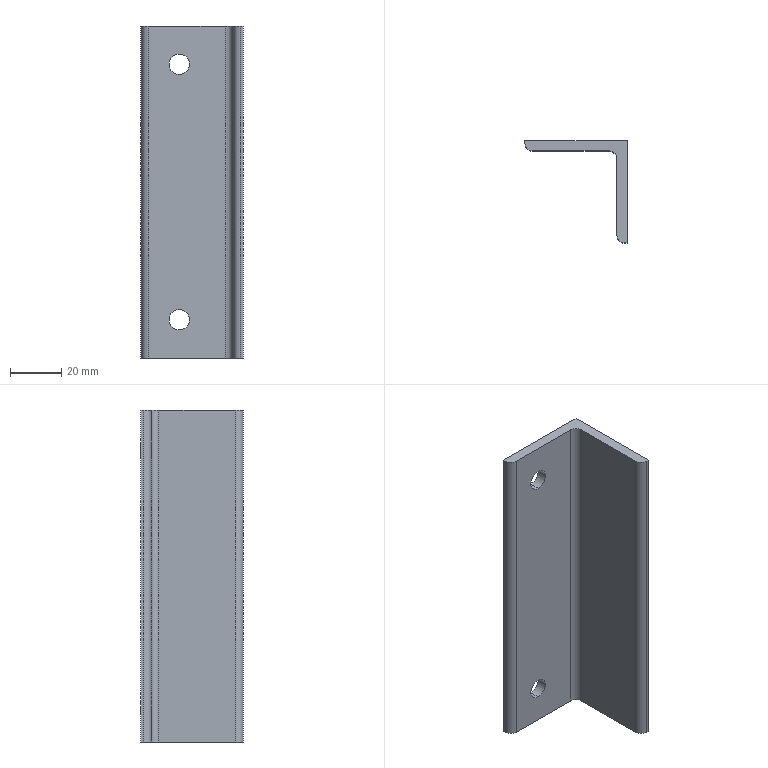Part | SolidWorks | features Extrusion 1, Fillet 1, ICE 1 | 1 solid | 15 faces | box 40 x 40 x 130 mm | volume 38867 mm3 | plane 8 | cylinder 7 | commonest cylinder face diameters 8 x4 6 x3
STEP:
#1=CARTESIAN_POINT('',(15.,0.,111.));
#2=VERTEX_POINT('',#1);
#3=CARTESIAN_POINT('',(15.,0.,119.));
#4=VERTEX_POINT('',#3);
#5=CARTESIAN_POINT('',(15.,0.,115.));
#6=DIRECTION('',(0.,1.,0.));
#7=DIRECTION('',(0.,0.,1.));
#8=AXIS2_PLACEMENT_3D('',#5,#6,#7);
#9=CIRCLE('',#8,4.);
#10=EDGE_CURVE('',#2,#4,#9,.T.);
#11=ORIENTED_EDGE('',*,*,#10,.T.);
#12=CARTESIAN_POINT('',(15.,-4.,119.));
#13=VERTEX_POINT('',#12);
#14=CARTESIAN_POINT('',(15.,126.,119.));
#15=DIRECTION('',(0.,-1.,0.));
#16=VECTOR('',#15,1000.);
#17=LINE('',#14,#16);
#18=EDGE_CURVE('',#4,#13,#17,.T.);
#19=ORIENTED_EDGE('',*,*,#18,.T.);
#20=CARTESIAN_POINT('',(15.,-4.,111.));
#21=VERTEX_POINT('',#20);
#22=CARTESIAN_POINT('',(15.,-4.,115.));
#23=DIRECTION('',(0.,-1.,0.));
#24=DIRECTION('',(0.,0.,-1.));
#25=AXIS2_PLACEMENT_3D('',#22,#23,#24);
#26=CIRCLE('',#25,4.);
#27=EDGE_CURVE('',#13,#21,#26,.T.);
#28=ORIENTED_EDGE('',*,*,#27,.T.);
#29=CARTESIAN_POINT('',(15.,126.,111.));
#30=DIRECTION('',(0.,-1.,0.));
#31=VECTOR('',#30,1000.);
#32=LINE('',#29,#31);
#33=EDGE_CURVE('',#2,#21,#32,.T.);
#34=ORIENTED_EDGE('',*,*,#33,.F.);
#35=EDGE_LOOP('',(#11,#19,#28,#34));
#36=FACE_OUTER_BOUND('',#35,.T.);
#37=CARTESIAN_POINT('',(15.,126.,115.));
#38=DIRECTION('',(0.,-1.,0.));
#39=DIRECTION('',(0.,0.,-1.));
#40=AXIS2_PLACEMENT_3D('',#37,#38,#39);
#41=CYLINDRICAL_SURFACE('',#40,4.);
#42=ADVANCED_FACE('',(#36),#41,.F.);
#43=CARTESIAN_POINT('',(15.,0.,11.));
#44=VERTEX_POINT('',#43);
#45=CARTESIAN_POINT('',(15.,0.,19.));
#46=VERTEX_POINT('',#45);
#47=CARTESIAN_POINT('',(15.,0.,15.));
#48=DIRECTION('',(0.,1.,0.));
#49=DIRECTION('',(0.,0.,1.));
#50=AXIS2_PLACEMENT_3D('',#47,#48,#49);
#51=CIRCLE('',#50,4.);
#52=EDGE_CURVE('',#44,#46,#51,.T.);
#53=ORIENTED_EDGE('',*,*,#52,.T.);
#54=CARTESIAN_POINT('',(15.,-4.,19.));
#55=VERTEX_POINT('',#54);
#56=CARTESIAN_POINT('',(15.,126.,19.));
#57=DIRECTION('',(0.,-1.,0.));
#58=VECTOR('',#57,1000.);
#59=LINE('',#56,#58);
#60=EDGE_CURVE('',#46,#55,#59,.T.);
#61=ORIENTED_EDGE('',*,*,#60,.T.);
#62=CARTESIAN_POINT('',(15.,-4.,11.));
#63=VERTEX_POINT('',#62);
#64=CARTESIAN_POINT('',(15.,-4.,15.));
#65=DIRECTION('',(0.,-1.,0.));
#66=DIRECTION('',(0.,0.,-1.));
#67=AXIS2_PLACEMENT_3D('',#64,#65,#66);
#68=CIRCLE('',#67,4.);
#69=EDGE_CURVE('',#55,#63,#68,.T.);
#70=ORIENTED_EDGE('',*,*,#69,.T.);
#71=CARTESIAN_POINT('',(15.,126.,11.));
#72=DIRECTION('',(0.,-1.,0.));
#73=VECTOR('',#72,1000.);
#74=LINE('',#71,#73);
#75=EDGE_CURVE('',#44,#63,#74,.T.);
#76=ORIENTED_EDGE('',*,*,#75,.F.);
#77=EDGE_LOOP('',(#53,#61,#70,#76));
#78=FACE_OUTER_BOUND('',#77,.T.);
#79=CARTESIAN_POINT('',(15.,126.,15.));
#80=DIRECTION('',(0.,-1.,0.));
#81=DIRECTION('',(0.,0.,-1.));
#82=AXIS2_PLACEMENT_3D('',#79,#80,#81);
#83=CYLINDRICAL_SURFACE('',#82,4.);
#84=ADVANCED_FACE('',(#78),#83,.F.);
#85=CARTESIAN_POINT('',(40.,0.,0.));
#86=VERTEX_POINT('',#85);
#87=CARTESIAN_POINT('',(40.,-40.,0.));
#88=VERTEX_POINT('',#87);
#89=CARTESIAN_POINT('',(40.,0.,0.));
#90=DIRECTION('',(0.,-1.,0.));
#91=VECTOR('',#90,1000.);
#92=LINE('',#89,#91);
#93=EDGE_CURVE('',#86,#88,#92,.T.);
#94=ORIENTED_EDGE('',*,*,#93,.F.);
#95=CARTESIAN_POINT('',(40.,0.,130.));
#96=VERTEX_POINT('',#95);
#97=CARTESIAN_POINT('',(40.,0.,130.));
#98=DIRECTION('',(0.,0.,-1.));
#99=VECTOR('',#98,1000.);
#100=LINE('',#97,#99);
#101=EDGE_CURVE('',#96,#86,#100,.T.);
#102=ORIENTED_EDGE('',*,*,#101,.F.);
#103=CARTESIAN_POINT('',(40.,-40.,130.));
#104=VERTEX_POINT('',#103);
#105=CARTESIAN_POINT('',(40.,0.,130.));
#106=DIRECTION('',(0.,-1.,0.));
#107=VECTOR('',#106,1000.);
#108=LINE('',#105,#107);
#109=EDGE_CURVE('',#96,#104,#108,.T.);
#110=ORIENTED_EDGE('',*,*,#109,.T.);
#111=CARTESIAN_POINT('',(40.,-40.,130.));
#112=DIRECTION('',(0.,0.,-1.));
#113=VECTOR('',#112,1000.);
#114=LINE('',#111,#113);
#115=EDGE_CURVE('',#104,#88,#114,.T.);
#116=ORIENTED_EDGE('',*,*,#115,.T.);
#117=EDGE_LOOP('',(#94,#102,#110,#116));
#118=FACE_OUTER_BOUND('',#117,.T.);
#119=CARTESIAN_POINT('',(40.,0.,130.));
#120=DIRECTION('',(1.,0.,0.));
#121=DIRECTION('',(0.,1.,0.));
#122=AXIS2_PLACEMENT_3D('',#119,#120,#121);
#123=PLANE('',#122);
#124=ADVANCED_FACE('',(#118),#123,.T.);
#125=ORIENTED_EDGE('',*,*,#10,.F.);
#126=CARTESIAN_POINT('',(15.,0.,115.));
#127=DIRECTION('',(0.,1.,0.));
#128=DIRECTION('',(0.,0.,1.));
#129=AXIS2_PLACEMENT_3D('',#126,#127,#128);
#130=CIRCLE('',#129,4.);
#131=EDGE_CURVE('',#4,#2,#130,.T.);
#132=ORIENTED_EDGE('',*,*,#131,.F.);
#133=EDGE_LOOP('',(#125,#132));
#134=FACE_BOUND('',#133,.T.);
#135=ORIENTED_EDGE('',*,*,#52,.F.);
#136=CARTESIAN_POINT('',(15.,0.,15.));
#137=DIRECTION('',(0.,1.,0.));
#138=DIRECTION('',(0.,0.,1.));
#139=AXIS2_PLACEMENT_3D('',#136,#137,#138);
#140=CIRCLE('',#139,4.);
#141=EDGE_CURVE('',#46,#44,#140,.T.);
#142=ORIENTED_EDGE('',*,*,#141,.F.);
#143=EDGE_LOOP('',(#135,#142));
#144=FACE_BOUND('',#143,.T.);
#145=CARTESIAN_POINT('',(0.,0.,0.));
#146=VERTEX_POINT('',#145);
#147=CARTESIAN_POINT('',(0.,0.,0.));
#148=DIRECTION('',(1.,0.,0.));
#149=VECTOR('',#148,1000.);
#150=LINE('',#147,#149);
#151=EDGE_CURVE('',#146,#86,#150,.T.);
#152=ORIENTED_EDGE('',*,*,#151,.F.);
#153=CARTESIAN_POINT('',(0.,0.,130.));
#154=VERTEX_POINT('',#153);
#155=CARTESIAN_POINT('',(0.,0.,130.));
#156=DIRECTION('',(0.,0.,-1.));
#157=VECTOR('',#156,1000.);
#158=LINE('',#155,#157);
#159=EDGE_CURVE('',#154,#146,#158,.T.);
#160=ORIENTED_EDGE('',*,*,#159,.F.);
#161=CARTESIAN_POINT('',(0.,0.,130.));
#162=DIRECTION('',(1.,0.,0.));
#163=VECTOR('',#162,1000.);
#164=LINE('',#161,#163);
#165=EDGE_CURVE('',#154,#96,#164,.T.);
#166=ORIENTED_EDGE('',*,*,#165,.T.);
#167=ORIENTED_EDGE('',*,*,#101,.T.);
#168=EDGE_LOOP('',(#152,#160,#166,#167));
#169=FACE_OUTER_BOUND('',#168,.T.);
#170=CARTESIAN_POINT('',(0.,0.,130.));
#171=DIRECTION('',(0.,1.,0.));
#172=DIRECTION('',(0.,0.,1.));
#173=AXIS2_PLACEMENT_3D('',#170,#171,#172);
#174=PLANE('',#173);
#175=ADVANCED_FACE('',(#134,#144,#169),#174,.T.);
#176=CARTESIAN_POINT('',(0.,-1.,0.));
#177=VERTEX_POINT('',#176);
#178=CARTESIAN_POINT('',(0.,0.,0.));
#179=DIRECTION('',(0.,-1.,0.));
#180=VECTOR('',#179,1000.);
#181=LINE('',#178,#180);
#182=EDGE_CURVE('',#146,#177,#181,.T.);
#183=ORIENTED_EDGE('',*,*,#182,.T.);
#184=CARTESIAN_POINT('',(0.,-1.,130.));
#185=VERTEX_POINT('',#184);
#186=CARTESIAN_POINT('',(0.,-1.,130.));
#187=DIRECTION('',(0.,0.,1.));
#188=VECTOR('',#187,1000.);
#189=LINE('',#186,#188);
#190=EDGE_CURVE('',#177,#185,#189,.T.);
#191=ORIENTED_EDGE('',*,*,#190,.T.);
#192=CARTESIAN_POINT('',(0.,0.,130.));
#193=DIRECTION('',(0.,-1.,0.));
#194=VECTOR('',#193,1000.);
#195=LINE('',#192,#194);
#196=EDGE_CURVE('',#154,#185,#195,.T.);
#197=ORIENTED_EDGE('',*,*,#196,.F.);
#198=ORIENTED_EDGE('',*,*,#159,.T.);
#199=EDGE_LOOP('',(#183,#191,#197,#198));
#200=FACE_OUTER_BOUND('',#199,.T.);
#201=CARTESIAN_POINT('',(0.,0.,130.));
#202=DIRECTION('',(1.,0.,0.));
#203=DIRECTION('',(0.,0.,-1.));
#204=AXIS2_PLACEMENT_3D('',#201,#202,#203);
#205=PLANE('',#204);
#206=ADVANCED_FACE('',(#200),#205,.F.);
#207=CARTESIAN_POINT('',(15.,-4.,115.));
#208=DIRECTION('',(0.,-1.,0.));
#209=DIRECTION('',(0.,0.,-1.));
#210=AXIS2_PLACEMENT_3D('',#207,#208,#209);
#211=CIRCLE('',#210,4.);
#212=EDGE_CURVE('',#21,#13,#211,.T.);
#213=ORIENTED_EDGE('',*,*,#212,.F.);
#214=ORIENTED_EDGE('',*,*,#27,.F.);
#215=EDGE_LOOP('',(#213,#214));
#216=FACE_BOUND('',#215,.T.);
#217=CARTESIAN_POINT('',(15.,-4.,15.));
#218=DIRECTION('',(0.,-1.,0.));
#219=DIRECTION('',(0.,0.,-1.));
#220=AXIS2_PLACEMENT_3D('',#217,#218,#219);
#221=CIRCLE('',#220,4.);
#222=EDGE_CURVE('',#63,#55,#221,.T.);
#223=ORIENTED_EDGE('',*,*,#222,.F.);
#224=ORIENTED_EDGE('',*,*,#69,.F.);
#225=EDGE_LOOP('',(#223,#224));
#226=FACE_BOUND('',#225,.T.);
#227=CARTESIAN_POINT('',(3.,-4.,0.));
#228=VERTEX_POINT('',#227);
#229=CARTESIAN_POINT('',(33.,-4.,0.));
#230=VERTEX_POINT('',#229);
#231=CARTESIAN_POINT('',(0.,-4.,0.));
#232=DIRECTION('',(1.,0.,0.));
#233=VECTOR('',#232,1000.);
#234=LINE('',#231,#233);
#235=EDGE_CURVE('',#228,#230,#234,.T.);
#236=ORIENTED_EDGE('',*,*,#235,.T.);
#237=CARTESIAN_POINT('',(33.,-4.,130.));
#238=VERTEX_POINT('',#237);
#239=CARTESIAN_POINT('',(33.,-4.,130.));
#240=DIRECTION('',(0.,0.,1.));
#241=VECTOR('',#240,1000.);
#242=LINE('',#239,#241);
#243=EDGE_CURVE('',#230,#238,#242,.T.);
#244=ORIENTED_EDGE('',*,*,#243,.T.);
#245=CARTESIAN_POINT('',(3.,-4.,130.));
#246=VERTEX_POINT('',#245);
#247=CARTESIAN_POINT('',(0.,-4.,130.));
#248=DIRECTION('',(1.,0.,0.));
#249=VECTOR('',#248,1000.);
#250=LINE('',#247,#249);
#251=EDGE_CURVE('',#246,#238,#250,.T.);
#252=ORIENTED_EDGE('',*,*,#251,.F.);
#253=CARTESIAN_POINT('',(3.,-4.,130.));
#254=DIRECTION('',(0.,0.,-1.));
#255=VECTOR('',#254,1000.);
#256=LINE('',#253,#255);
#257=EDGE_CURVE('',#246,#228,#256,.T.);
#258=ORIENTED_EDGE('',*,*,#257,.T.);
#259=EDGE_LOOP('',(#236,#244,#252,#258));
#260=FACE_OUTER_BOUND('',#259,.T.);
#261=CARTESIAN_POINT('',(0.,-4.,130.));
#262=DIRECTION('',(0.,1.,0.));
#263=DIRECTION('',(0.,0.,1.));
#264=AXIS2_PLACEMENT_3D('',#261,#262,#263);
#265=PLANE('',#264);
#266=ADVANCED_FACE('',(#216,#226,#260),#265,.F.);
#267=CARTESIAN_POINT('',(36.,-7.,130.));
#268=VERTEX_POINT('',#267);
#269=CARTESIAN_POINT('',(36.,-37.,130.));
#270=VERTEX_POINT('',#269);
#271=CARTESIAN_POINT('',(36.,-4.,130.));
#272=DIRECTION('',(0.,-1.,0.));
#273=VECTOR('',#272,1000.);
#274=LINE('',#271,#273);
#275=EDGE_CURVE('',#268,#270,#274,.T.);
#276=ORIENTED_EDGE('',*,*,#275,.F.);
#277=CARTESIAN_POINT('',(36.,-7.,0.));
#278=VERTEX_POINT('',#277);
#279=CARTESIAN_POINT('',(36.,-7.,0.));
#280=DIRECTION('',(0.,0.,-1.));
#281=VECTOR('',#280,1000.);
#282=LINE('',#279,#281);
#283=EDGE_CURVE('',#268,#278,#282,.T.);
#284=ORIENTED_EDGE('',*,*,#283,.T.);
#285=CARTESIAN_POINT('',(36.,-37.,0.));
#286=VERTEX_POINT('',#285);
#287=CARTESIAN_POINT('',(36.,-4.,0.));
#288=DIRECTION('',(0.,-1.,0.));
#289=VECTOR('',#288,1000.);
#290=LINE('',#287,#289);
#291=EDGE_CURVE('',#278,#286,#290,.T.);
#292=ORIENTED_EDGE('',*,*,#291,.T.);
#293=CARTESIAN_POINT('',(36.,-37.,130.));
#294=DIRECTION('',(0.,0.,1.));
#295=VECTOR('',#294,1000.);
#296=LINE('',#293,#295);
#297=EDGE_CURVE('',#286,#270,#296,.T.);
#298=ORIENTED_EDGE('',*,*,#297,.T.);
#299=EDGE_LOOP('',(#276,#284,#292,#298));
#300=FACE_OUTER_BOUND('',#299,.T.);
#301=CARTESIAN_POINT('',(36.,-4.,130.));
#302=DIRECTION('',(1.,0.,0.));
#303=DIRECTION('',(0.,0.,-1.));
#304=AXIS2_PLACEMENT_3D('',#301,#302,#303);
#305=PLANE('',#304);
#306=ADVANCED_FACE('',(#300),#305,.F.);
#307=CARTESIAN_POINT('',(39.,-40.,130.));
#308=VERTEX_POINT('',#307);
#309=CARTESIAN_POINT('',(40.,-40.,130.));
#310=DIRECTION('',(-1.,0.,0.));
#311=VECTOR('',#310,1000.);
#312=LINE('',#309,#311);
#313=EDGE_CURVE('',#104,#308,#312,.T.);
#314=ORIENTED_EDGE('',*,*,#313,.T.);
#315=CARTESIAN_POINT('',(39.,-40.,0.));
#316=VERTEX_POINT('',#315);
#317=CARTESIAN_POINT('',(39.,-40.,0.));
#318=DIRECTION('',(0.,0.,-1.));
#319=VECTOR('',#318,1000.);
#320=LINE('',#317,#319);
#321=EDGE_CURVE('',#308,#316,#320,.T.);
#322=ORIENTED_EDGE('',*,*,#321,.T.);
#323=CARTESIAN_POINT('',(40.,-40.,0.));
#324=DIRECTION('',(-1.,0.,0.));
#325=VECTOR('',#324,1000.);
#326=LINE('',#323,#325);
#327=EDGE_CURVE('',#88,#316,#326,.T.);
#328=ORIENTED_EDGE('',*,*,#327,.F.);
#329=ORIENTED_EDGE('',*,*,#115,.F.);
#330=EDGE_LOOP('',(#314,#322,#328,#329));
#331=FACE_OUTER_BOUND('',#330,.T.);
#332=CARTESIAN_POINT('',(40.,-40.,130.));
#333=DIRECTION('',(0.,-1.,0.));
#334=DIRECTION('',(0.,0.,-1.));
#335=AXIS2_PLACEMENT_3D('',#332,#333,#334);
#336=PLANE('',#335);
#337=ADVANCED_FACE('',(#331),#336,.T.);
#338=ORIENTED_EDGE('',*,*,#275,.T.);
#339=CARTESIAN_POINT('',(39.,-37.,130.));
#340=DIRECTION('',(0.,0.,1.));
#341=DIRECTION('',(-1.,0.,0.));
#342=AXIS2_PLACEMENT_3D('',#339,#340,#341);
#343=CIRCLE('',#342,3.);
#344=EDGE_CURVE('',#270,#308,#343,.T.);
#345=ORIENTED_EDGE('',*,*,#344,.T.);
#346=ORIENTED_EDGE('',*,*,#313,.F.);
#347=ORIENTED_EDGE('',*,*,#109,.F.);
#348=ORIENTED_EDGE('',*,*,#165,.F.);
#349=ORIENTED_EDGE('',*,*,#196,.T.);
#350=CARTESIAN_POINT('',(3.,-1.,130.));
#351=DIRECTION('',(0.,0.,1.));
#352=DIRECTION('',(-1.,0.,0.));
#353=AXIS2_PLACEMENT_3D('',#350,#351,#352);
#354=CIRCLE('',#353,3.);
#355=EDGE_CURVE('',#185,#246,#354,.T.);
#356=ORIENTED_EDGE('',*,*,#355,.T.);
#357=ORIENTED_EDGE('',*,*,#251,.T.);
#358=CARTESIAN_POINT('',(33.,-7.,130.));
#359=DIRECTION('',(0.,0.,-1.));
#360=DIRECTION('',(-1.,0.,0.));
#361=AXIS2_PLACEMENT_3D('',#358,#359,#360);
#362=CIRCLE('',#361,3.);
#363=EDGE_CURVE('',#238,#268,#362,.T.);
#364=ORIENTED_EDGE('',*,*,#363,.T.);
#365=EDGE_LOOP('',(#338,#345,#346,#347,#348,#349,#356,#357,#364));
#366=FACE_OUTER_BOUND('',#365,.T.);
#367=CARTESIAN_POINT('',(0.,0.,130.));
#368=DIRECTION('',(0.,0.,-1.));
#369=DIRECTION('',(-1.,0.,0.));
#370=AXIS2_PLACEMENT_3D('',#367,#368,#369);
#371=PLANE('',#370);
#372=ADVANCED_FACE('',(#366),#371,.F.);
#373=ORIENTED_EDGE('',*,*,#327,.T.);
#374=CARTESIAN_POINT('',(39.,-37.,0.));
#375=DIRECTION('',(0.,0.,-1.));
#376=DIRECTION('',(-1.,0.,0.));
#377=AXIS2_PLACEMENT_3D('',#374,#375,#376);
#378=CIRCLE('',#377,3.);
#379=EDGE_CURVE('',#316,#286,#378,.T.);
#380=ORIENTED_EDGE('',*,*,#379,.T.);
#381=ORIENTED_EDGE('',*,*,#291,.F.);
#382=CARTESIAN_POINT('',(33.,-7.,0.));
#383=DIRECTION('',(0.,0.,1.));
#384=DIRECTION('',(-1.,0.,0.));
#385=AXIS2_PLACEMENT_3D('',#382,#383,#384);
#386=CIRCLE('',#385,3.);
#387=EDGE_CURVE('',#278,#230,#386,.T.);
#388=ORIENTED_EDGE('',*,*,#387,.T.);
#389=ORIENTED_EDGE('',*,*,#235,.F.);
#390=CARTESIAN_POINT('',(3.,-1.,0.));
#391=DIRECTION('',(0.,0.,-1.));
#392=DIRECTION('',(-1.,0.,0.));
#393=AXIS2_PLACEMENT_3D('',#390,#391,#392);
#394=CIRCLE('',#393,3.);
#395=EDGE_CURVE('',#228,#177,#394,.T.);
#396=ORIENTED_EDGE('',*,*,#395,.T.);
#397=ORIENTED_EDGE('',*,*,#182,.F.);
#398=ORIENTED_EDGE('',*,*,#151,.T.);
#399=ORIENTED_EDGE('',*,*,#93,.T.);
#400=EDGE_LOOP('',(#373,#380,#381,#388,#389,#396,#397,#398,#399));
#401=FACE_OUTER_BOUND('',#400,.T.);
#402=CARTESIAN_POINT('',(0.,0.,0.));
#403=DIRECTION('',(0.,0.,-1.));
#404=DIRECTION('',(-1.,0.,0.));
#405=AXIS2_PLACEMENT_3D('',#402,#403,#404);
#406=PLANE('',#405);
#407=ADVANCED_FACE('',(#401),#406,.T.);
#408=ORIENTED_EDGE('',*,*,#363,.F.);
#409=ORIENTED_EDGE('',*,*,#243,.F.);
#410=ORIENTED_EDGE('',*,*,#387,.F.);
#411=ORIENTED_EDGE('',*,*,#283,.F.);
#412=EDGE_LOOP('',(#408,#409,#410,#411));
#413=FACE_OUTER_BOUND('',#412,.T.);
#414=CARTESIAN_POINT('',(33.,-7.,130.));
#415=DIRECTION('',(0.,0.,1.));
#416=DIRECTION('',(1.,0.,0.));
#417=AXIS2_PLACEMENT_3D('',#414,#415,#416);
#418=CYLINDRICAL_SURFACE('',#417,3.);
#419=ADVANCED_FACE('',(#413),#418,.F.);
#420=ORIENTED_EDGE('',*,*,#344,.F.);
#421=ORIENTED_EDGE('',*,*,#297,.F.);
#422=ORIENTED_EDGE('',*,*,#379,.F.);
#423=ORIENTED_EDGE('',*,*,#321,.F.);
#424=EDGE_LOOP('',(#420,#421,#422,#423));
#425=FACE_OUTER_BOUND('',#424,.T.);
#426=CARTESIAN_POINT('',(39.,-37.,130.));
#427=DIRECTION('',(0.,0.,1.));
#428=DIRECTION('',(1.,0.,0.));
#429=AXIS2_PLACEMENT_3D('',#426,#427,#428);
#430=CYLINDRICAL_SURFACE('',#429,3.);
#431=ADVANCED_FACE('',(#425),#430,.T.);
#432=ORIENTED_EDGE('',*,*,#355,.F.);
#433=ORIENTED_EDGE('',*,*,#190,.F.);
#434=ORIENTED_EDGE('',*,*,#395,.F.);
#435=ORIENTED_EDGE('',*,*,#257,.F.);
#436=EDGE_LOOP('',(#432,#433,#434,#435));
#437=FACE_OUTER_BOUND('',#436,.T.);
#438=CARTESIAN_POINT('',(3.,-1.,130.));
#439=DIRECTION('',(0.,0.,-1.));
#440=DIRECTION('',(-1.,0.,0.));
#441=AXIS2_PLACEMENT_3D('',#438,#439,#440);
#442=CYLINDRICAL_SURFACE('',#441,3.);
#443=ADVANCED_FACE('',(#437),#442,.T.);
#444=ORIENTED_EDGE('',*,*,#60,.F.);
#445=ORIENTED_EDGE('',*,*,#141,.T.);
#446=ORIENTED_EDGE('',*,*,#75,.T.);
#447=ORIENTED_EDGE('',*,*,#222,.T.);
#448=EDGE_LOOP('',(#444,#445,#446,#447));
#449=FACE_OUTER_BOUND('',#448,.T.);
#450=CARTESIAN_POINT('',(15.,126.,15.));
#451=DIRECTION('',(0.,-1.,0.));
#452=DIRECTION('',(0.,0.,-1.));
#453=AXIS2_PLACEMENT_3D('',#450,#451,#452);
#454=CYLINDRICAL_SURFACE('',#453,4.);
#455=ADVANCED_FACE('',(#449),#454,.F.);
#456=ORIENTED_EDGE('',*,*,#18,.F.);
#457=ORIENTED_EDGE('',*,*,#131,.T.);
#458=ORIENTED_EDGE('',*,*,#33,.T.);
#459=ORIENTED_EDGE('',*,*,#212,.T.);
#460=EDGE_LOOP('',(#456,#457,#458,#459));
#461=FACE_OUTER_BOUND('',#460,.T.);
#462=CARTESIAN_POINT('',(15.,126.,115.));
#463=DIRECTION('',(0.,-1.,0.));
#464=DIRECTION('',(0.,0.,-1.));
#465=AXIS2_PLACEMENT_3D('',#462,#463,#464);
#466=CYLINDRICAL_SURFACE('',#465,4.);
#467=ADVANCED_FACE('',(#461),#466,.F.);
#468=CLOSED_SHELL('',(#42,#84,#124,#175,#206,#266,#306,#337,#372,#407,#419,#431,#443,#455,#467));
#469=MANIFOLD_SOLID_BREP('',#468);
#470=CARTESIAN_POINT('',(0.,0.,0.));
#471=DIRECTION('',(0.,0.,1.));
#472=DIRECTION('',(1.,0.,0.));
#473=AXIS2_PLACEMENT_3D('',#470,#471,#472);
#474=(LENGTH_UNIT()NAMED_UNIT(*)SI_UNIT(.MILLI.,.METRE.));
#475=UNCERTAINTY_MEASURE_WITH_UNIT(LENGTH_MEASURE(0.00001),#474,'','');
#476=(NAMED_UNIT(*)PLANE_ANGLE_UNIT()SI_UNIT($,.RADIAN.));
#477=(NAMED_UNIT(*)SI_UNIT($,.STERADIAN.)SOLID_ANGLE_UNIT());
#478=(GEOMETRIC_REPRESENTATION_CONTEXT(3)GLOBAL_UNCERTAINTY_ASSIGNED_CONTEXT((#475))GLOBAL_UNIT_ASSIGNED_CONTEXT((#474,#476,#477))REPRESENTATION_CONTEXT('',''));
#479=ADVANCED_BREP_SHAPE_REPRESENTATION('',(#469,#473),#478);